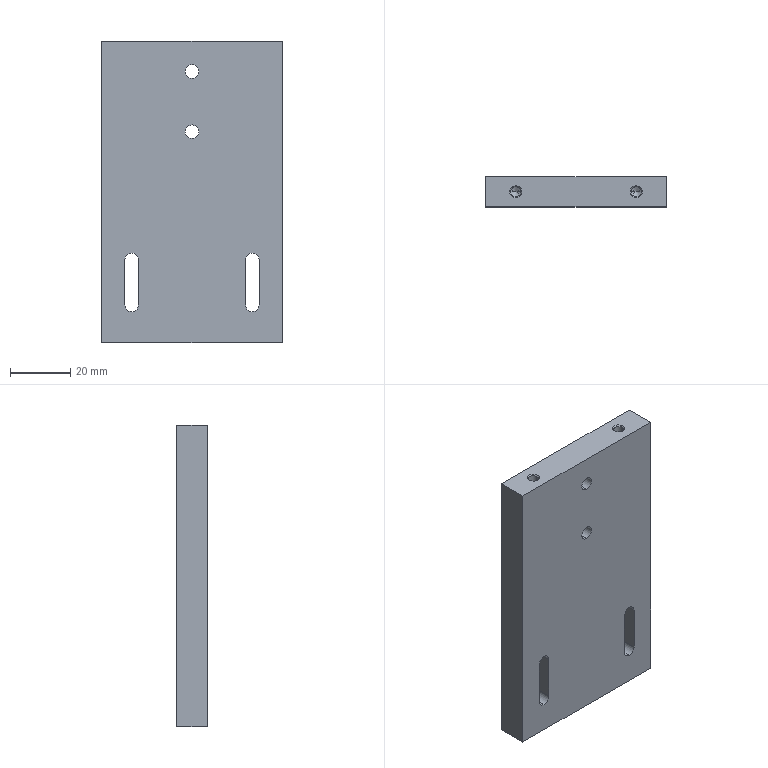Part | STEP file | Camera mounting upright plate | 1 solid | 44 faces | box 60 x 10 x 100 mm | volume 50291 mm3 | cylinder 20 | plane 16 | cone 8 | commonest cylinder face diameters 4.5 x10 3.3 x4 8 x4 10 x2